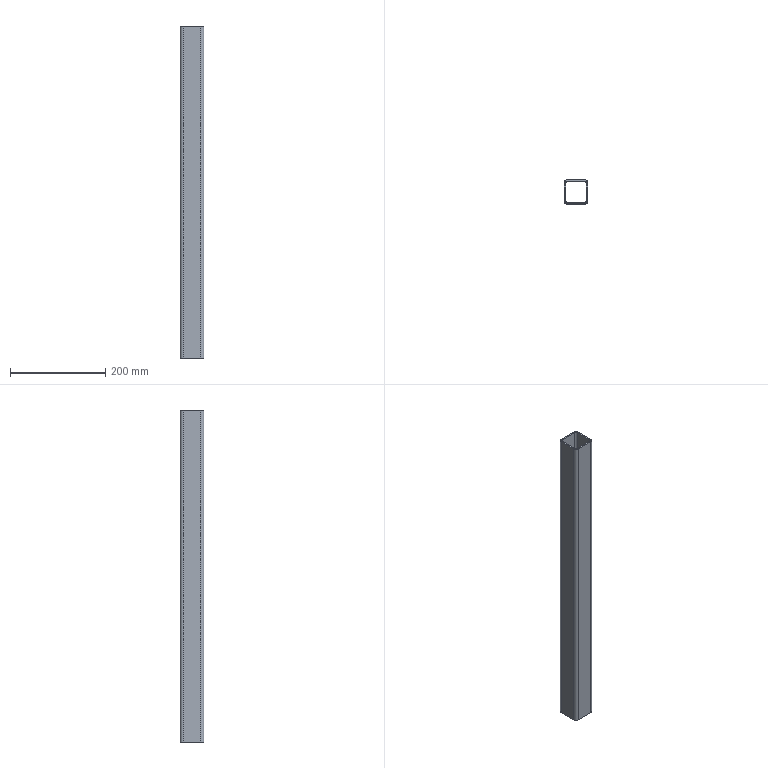Part | STEP file | JIS G 3466 50 x 50 x 3,2 1784904005805 | 1 solid | 18 faces | box 50 x 50 x 698.813 mm | volume 400189 mm3 | plane 10 | cylinder 8 | commonest cylinder face diameters 6.4 x4 12.8 x4
STEP:
#1=CARTESIAN_POINT('',(-18.6,-21.8,698.813));
#2=VERTEX_POINT('',#1);
#3=CARTESIAN_POINT('',(18.6,-21.8,698.813));
#4=VERTEX_POINT('',#3);
#5=CARTESIAN_POINT('',(9.3,-21.8,698.813));
#6=DIRECTION('',(1.,0.,0.));
#7=VECTOR('',#6,10.);
#8=LINE('',#5,#7);
#9=EDGE_CURVE('',#2,#4,#8,.T.);
#10=ORIENTED_EDGE('',*,*,#9,.T.);
#11=CARTESIAN_POINT('',(18.6,-21.8,0.));
#12=VERTEX_POINT('',#11);
#13=CARTESIAN_POINT('',(18.6,-21.8,0.));
#14=DIRECTION('',(0.,0.,1.));
#15=VECTOR('',#14,10.);
#16=LINE('',#13,#15);
#17=EDGE_CURVE('',#12,#4,#16,.T.);
#18=ORIENTED_EDGE('',*,*,#17,.F.);
#19=CARTESIAN_POINT('',(-18.6,-21.8,0.));
#20=VERTEX_POINT('',#19);
#21=CARTESIAN_POINT('',(9.3,-21.8,0.));
#22=DIRECTION('',(1.,0.,0.));
#23=VECTOR('',#22,10.);
#24=LINE('',#21,#23);
#25=EDGE_CURVE('',#20,#12,#24,.T.);
#26=ORIENTED_EDGE('',*,*,#25,.F.);
#27=CARTESIAN_POINT('',(-18.6,-21.8,0.));
#28=DIRECTION('',(0.,0.,1.));
#29=VECTOR('',#28,10.);
#30=LINE('',#27,#29);
#31=EDGE_CURVE('',#20,#2,#30,.T.);
#32=ORIENTED_EDGE('',*,*,#31,.T.);
#33=EDGE_LOOP('',(#10,#18,#26,#32));
#34=FACE_OUTER_BOUND('',#33,.T.);
#35=CARTESIAN_POINT('',(18.6,-21.8,0.));
#36=DIRECTION('',(0.,-1.,0.));
#37=DIRECTION('',(0.,0.,-1.));
#38=AXIS2_PLACEMENT_3D('',#35,#36,#37);
#39=PLANE('',#38);
#40=ADVANCED_FACE('',(#34),#39,.F.);
#41=CARTESIAN_POINT('',(21.8,-18.6,698.813));
#42=VERTEX_POINT('',#41);
#43=CARTESIAN_POINT('',(18.6,-18.6,698.813));
#44=DIRECTION('',(0.,0.,1.));
#45=DIRECTION('',(0.,1.,0.));
#46=AXIS2_PLACEMENT_3D('',#43,#44,#45);
#47=CIRCLE('',#46,3.2);
#48=EDGE_CURVE('',#4,#42,#47,.T.);
#49=ORIENTED_EDGE('',*,*,#48,.T.);
#50=CARTESIAN_POINT('',(21.8,-18.6,0.));
#51=VERTEX_POINT('',#50);
#52=CARTESIAN_POINT('',(21.8,-18.6,0.));
#53=DIRECTION('',(0.,0.,1.));
#54=VECTOR('',#53,10.);
#55=LINE('',#52,#54);
#56=EDGE_CURVE('',#51,#42,#55,.T.);
#57=ORIENTED_EDGE('',*,*,#56,.F.);
#58=CARTESIAN_POINT('',(18.6,-18.6,0.));
#59=DIRECTION('',(0.,0.,1.));
#60=DIRECTION('',(0.,1.,0.));
#61=AXIS2_PLACEMENT_3D('',#58,#59,#60);
#62=CIRCLE('',#61,3.2);
#63=EDGE_CURVE('',#12,#51,#62,.T.);
#64=ORIENTED_EDGE('',*,*,#63,.F.);
#65=ORIENTED_EDGE('',*,*,#17,.T.);
#66=EDGE_LOOP('',(#49,#57,#64,#65));
#67=FACE_OUTER_BOUND('',#66,.T.);
#68=CARTESIAN_POINT('',(18.6,-18.6,0.));
#69=DIRECTION('',(0.,0.,1.));
#70=DIRECTION('',(0.,1.,0.));
#71=AXIS2_PLACEMENT_3D('',#68,#69,#70);
#72=CYLINDRICAL_SURFACE('',#71,3.2);
#73=ADVANCED_FACE('',(#67),#72,.F.);
#74=CARTESIAN_POINT('',(21.8,18.6,698.813));
#75=VERTEX_POINT('',#74);
#76=CARTESIAN_POINT('',(21.8,9.3,698.813));
#77=DIRECTION('',(0.,1.,0.));
#78=VECTOR('',#77,10.);
#79=LINE('',#76,#78);
#80=EDGE_CURVE('',#42,#75,#79,.T.);
#81=ORIENTED_EDGE('',*,*,#80,.T.);
#82=CARTESIAN_POINT('',(21.8,18.6,0.));
#83=VERTEX_POINT('',#82);
#84=CARTESIAN_POINT('',(21.8,18.6,0.));
#85=DIRECTION('',(0.,0.,1.));
#86=VECTOR('',#85,10.);
#87=LINE('',#84,#86);
#88=EDGE_CURVE('',#83,#75,#87,.T.);
#89=ORIENTED_EDGE('',*,*,#88,.F.);
#90=CARTESIAN_POINT('',(21.8,9.3,0.));
#91=DIRECTION('',(0.,1.,0.));
#92=VECTOR('',#91,10.);
#93=LINE('',#90,#92);
#94=EDGE_CURVE('',#51,#83,#93,.T.);
#95=ORIENTED_EDGE('',*,*,#94,.F.);
#96=ORIENTED_EDGE('',*,*,#56,.T.);
#97=EDGE_LOOP('',(#81,#89,#95,#96));
#98=FACE_OUTER_BOUND('',#97,.T.);
#99=CARTESIAN_POINT('',(21.8,18.6,0.));
#100=DIRECTION('',(1.,0.,0.));
#101=DIRECTION('',(0.,0.,-1.));
#102=AXIS2_PLACEMENT_3D('',#99,#100,#101);
#103=PLANE('',#102);
#104=ADVANCED_FACE('',(#98),#103,.F.);
#105=CARTESIAN_POINT('',(18.6,21.8,698.813));
#106=VERTEX_POINT('',#105);
#107=CARTESIAN_POINT('',(18.6,18.6,698.813));
#108=DIRECTION('',(0.,0.,1.));
#109=DIRECTION('',(-1.,0.,0.));
#110=AXIS2_PLACEMENT_3D('',#107,#108,#109);
#111=CIRCLE('',#110,3.2);
#112=EDGE_CURVE('',#75,#106,#111,.T.);
#113=ORIENTED_EDGE('',*,*,#112,.T.);
#114=CARTESIAN_POINT('',(18.6,21.8,0.));
#115=VERTEX_POINT('',#114);
#116=CARTESIAN_POINT('',(18.6,21.8,0.));
#117=DIRECTION('',(0.,0.,1.));
#118=VECTOR('',#117,10.);
#119=LINE('',#116,#118);
#120=EDGE_CURVE('',#115,#106,#119,.T.);
#121=ORIENTED_EDGE('',*,*,#120,.F.);
#122=CARTESIAN_POINT('',(18.6,18.6,0.));
#123=DIRECTION('',(0.,0.,1.));
#124=DIRECTION('',(-1.,0.,0.));
#125=AXIS2_PLACEMENT_3D('',#122,#123,#124);
#126=CIRCLE('',#125,3.2);
#127=EDGE_CURVE('',#83,#115,#126,.T.);
#128=ORIENTED_EDGE('',*,*,#127,.F.);
#129=ORIENTED_EDGE('',*,*,#88,.T.);
#130=EDGE_LOOP('',(#113,#121,#128,#129));
#131=FACE_OUTER_BOUND('',#130,.T.);
#132=CARTESIAN_POINT('',(18.6,18.6,0.));
#133=DIRECTION('',(0.,0.,1.));
#134=DIRECTION('',(-1.,0.,0.));
#135=AXIS2_PLACEMENT_3D('',#132,#133,#134);
#136=CYLINDRICAL_SURFACE('',#135,3.2);
#137=ADVANCED_FACE('',(#131),#136,.F.);
#138=CARTESIAN_POINT('',(25.,18.6,698.813));
#139=VERTEX_POINT('',#138);
#140=CARTESIAN_POINT('',(25.,-18.6,698.813));
#141=VERTEX_POINT('',#140);
#142=CARTESIAN_POINT('',(25.,9.3,698.813));
#143=DIRECTION('',(0.,-1.,0.));
#144=VECTOR('',#143,10.);
#145=LINE('',#142,#144);
#146=EDGE_CURVE('',#139,#141,#145,.T.);
#147=ORIENTED_EDGE('',*,*,#146,.T.);
#148=CARTESIAN_POINT('',(25.,-18.6,0.));
#149=VERTEX_POINT('',#148);
#150=CARTESIAN_POINT('',(25.,-18.6,0.));
#151=DIRECTION('',(0.,0.,1.));
#152=VECTOR('',#151,10.);
#153=LINE('',#150,#152);
#154=EDGE_CURVE('',#149,#141,#153,.T.);
#155=ORIENTED_EDGE('',*,*,#154,.F.);
#156=CARTESIAN_POINT('',(25.,18.6,0.));
#157=VERTEX_POINT('',#156);
#158=CARTESIAN_POINT('',(25.,9.3,0.));
#159=DIRECTION('',(0.,-1.,0.));
#160=VECTOR('',#159,10.);
#161=LINE('',#158,#160);
#162=EDGE_CURVE('',#157,#149,#161,.T.);
#163=ORIENTED_EDGE('',*,*,#162,.F.);
#164=CARTESIAN_POINT('',(25.,18.6,0.));
#165=DIRECTION('',(0.,0.,1.));
#166=VECTOR('',#165,10.);
#167=LINE('',#164,#166);
#168=EDGE_CURVE('',#157,#139,#167,.T.);
#169=ORIENTED_EDGE('',*,*,#168,.T.);
#170=EDGE_LOOP('',(#147,#155,#163,#169));
#171=FACE_OUTER_BOUND('',#170,.T.);
#172=CARTESIAN_POINT('',(25.,18.6,0.));
#173=DIRECTION('',(1.,0.,0.));
#174=DIRECTION('',(0.,0.,-1.));
#175=AXIS2_PLACEMENT_3D('',#172,#173,#174);
#176=PLANE('',#175);
#177=ADVANCED_FACE('',(#171),#176,.T.);
#178=CARTESIAN_POINT('',(18.6,-25.,698.813));
#179=VERTEX_POINT('',#178);
#180=CARTESIAN_POINT('',(18.6,-18.6,698.813));
#181=DIRECTION('',(0.,0.,-1.));
#182=DIRECTION('',(0.,1.,0.));
#183=AXIS2_PLACEMENT_3D('',#180,#181,#182);
#184=CIRCLE('',#183,6.4);
#185=EDGE_CURVE('',#141,#179,#184,.T.);
#186=ORIENTED_EDGE('',*,*,#185,.T.);
#187=CARTESIAN_POINT('',(18.6,-25.,0.));
#188=VERTEX_POINT('',#187);
#189=CARTESIAN_POINT('',(18.6,-25.,0.));
#190=DIRECTION('',(0.,0.,1.));
#191=VECTOR('',#190,10.);
#192=LINE('',#189,#191);
#193=EDGE_CURVE('',#188,#179,#192,.T.);
#194=ORIENTED_EDGE('',*,*,#193,.F.);
#195=CARTESIAN_POINT('',(18.6,-18.6,0.));
#196=DIRECTION('',(0.,0.,-1.));
#197=DIRECTION('',(0.,1.,0.));
#198=AXIS2_PLACEMENT_3D('',#195,#196,#197);
#199=CIRCLE('',#198,6.4);
#200=EDGE_CURVE('',#149,#188,#199,.T.);
#201=ORIENTED_EDGE('',*,*,#200,.F.);
#202=ORIENTED_EDGE('',*,*,#154,.T.);
#203=EDGE_LOOP('',(#186,#194,#201,#202));
#204=FACE_OUTER_BOUND('',#203,.T.);
#205=CARTESIAN_POINT('',(18.6,-18.6,0.));
#206=DIRECTION('',(0.,0.,1.));
#207=DIRECTION('',(0.,1.,0.));
#208=AXIS2_PLACEMENT_3D('',#205,#206,#207);
#209=CYLINDRICAL_SURFACE('',#208,6.4);
#210=ADVANCED_FACE('',(#204),#209,.T.);
#211=CARTESIAN_POINT('',(-18.6,-25.,698.813));
#212=VERTEX_POINT('',#211);
#213=CARTESIAN_POINT('',(9.3,-25.,698.813));
#214=DIRECTION('',(-1.,0.,0.));
#215=VECTOR('',#214,10.);
#216=LINE('',#213,#215);
#217=EDGE_CURVE('',#179,#212,#216,.T.);
#218=ORIENTED_EDGE('',*,*,#217,.T.);
#219=CARTESIAN_POINT('',(-18.6,-25.,0.));
#220=VERTEX_POINT('',#219);
#221=CARTESIAN_POINT('',(-18.6,-25.,0.));
#222=DIRECTION('',(0.,0.,1.));
#223=VECTOR('',#222,10.);
#224=LINE('',#221,#223);
#225=EDGE_CURVE('',#220,#212,#224,.T.);
#226=ORIENTED_EDGE('',*,*,#225,.F.);
#227=CARTESIAN_POINT('',(9.3,-25.,0.));
#228=DIRECTION('',(-1.,0.,0.));
#229=VECTOR('',#228,10.);
#230=LINE('',#227,#229);
#231=EDGE_CURVE('',#188,#220,#230,.T.);
#232=ORIENTED_EDGE('',*,*,#231,.F.);
#233=ORIENTED_EDGE('',*,*,#193,.T.);
#234=EDGE_LOOP('',(#218,#226,#232,#233));
#235=FACE_OUTER_BOUND('',#234,.T.);
#236=CARTESIAN_POINT('',(18.6,-25.,0.));
#237=DIRECTION('',(0.,-1.,0.));
#238=DIRECTION('',(0.,0.,-1.));
#239=AXIS2_PLACEMENT_3D('',#236,#237,#238);
#240=PLANE('',#239);
#241=ADVANCED_FACE('',(#235),#240,.T.);
#242=CARTESIAN_POINT('',(-25.,-18.6,698.813));
#243=VERTEX_POINT('',#242);
#244=CARTESIAN_POINT('',(-18.6,-18.6,698.813));
#245=DIRECTION('',(0.,0.,-1.));
#246=DIRECTION('',(1.,0.,0.));
#247=AXIS2_PLACEMENT_3D('',#244,#245,#246);
#248=CIRCLE('',#247,6.4);
#249=EDGE_CURVE('',#212,#243,#248,.T.);
#250=ORIENTED_EDGE('',*,*,#249,.T.);
#251=CARTESIAN_POINT('',(-25.,-18.6,0.));
#252=VERTEX_POINT('',#251);
#253=CARTESIAN_POINT('',(-25.,-18.6,0.));
#254=DIRECTION('',(0.,0.,1.));
#255=VECTOR('',#254,10.);
#256=LINE('',#253,#255);
#257=EDGE_CURVE('',#252,#243,#256,.T.);
#258=ORIENTED_EDGE('',*,*,#257,.F.);
#259=CARTESIAN_POINT('',(-18.6,-18.6,0.));
#260=DIRECTION('',(0.,0.,-1.));
#261=DIRECTION('',(1.,0.,0.));
#262=AXIS2_PLACEMENT_3D('',#259,#260,#261);
#263=CIRCLE('',#262,6.4);
#264=EDGE_CURVE('',#220,#252,#263,.T.);
#265=ORIENTED_EDGE('',*,*,#264,.F.);
#266=ORIENTED_EDGE('',*,*,#225,.T.);
#267=EDGE_LOOP('',(#250,#258,#265,#266));
#268=FACE_OUTER_BOUND('',#267,.T.);
#269=CARTESIAN_POINT('',(-18.6,-18.6,0.));
#270=DIRECTION('',(0.,0.,1.));
#271=DIRECTION('',(1.,0.,0.));
#272=AXIS2_PLACEMENT_3D('',#269,#270,#271);
#273=CYLINDRICAL_SURFACE('',#272,6.4);
#274=ADVANCED_FACE('',(#268),#273,.T.);
#275=CARTESIAN_POINT('',(-18.6,21.8,698.813));
#276=VERTEX_POINT('',#275);
#277=CARTESIAN_POINT('',(-9.3,21.8,698.813));
#278=DIRECTION('',(-1.,0.,0.));
#279=VECTOR('',#278,10.);
#280=LINE('',#277,#279);
#281=EDGE_CURVE('',#106,#276,#280,.T.);
#282=ORIENTED_EDGE('',*,*,#281,.T.);
#283=CARTESIAN_POINT('',(-18.6,21.8,0.));
#284=VERTEX_POINT('',#283);
#285=CARTESIAN_POINT('',(-18.6,21.8,0.));
#286=DIRECTION('',(0.,0.,1.));
#287=VECTOR('',#286,10.);
#288=LINE('',#285,#287);
#289=EDGE_CURVE('',#284,#276,#288,.T.);
#290=ORIENTED_EDGE('',*,*,#289,.F.);
#291=CARTESIAN_POINT('',(-9.3,21.8,0.));
#292=DIRECTION('',(-1.,0.,0.));
#293=VECTOR('',#292,10.);
#294=LINE('',#291,#293);
#295=EDGE_CURVE('',#115,#284,#294,.T.);
#296=ORIENTED_EDGE('',*,*,#295,.F.);
#297=ORIENTED_EDGE('',*,*,#120,.T.);
#298=EDGE_LOOP('',(#282,#290,#296,#297));
#299=FACE_OUTER_BOUND('',#298,.T.);
#300=CARTESIAN_POINT('',(-18.6,21.8,0.));
#301=DIRECTION('',(0.,1.,0.));
#302=DIRECTION('',(0.,0.,1.));
#303=AXIS2_PLACEMENT_3D('',#300,#301,#302);
#304=PLANE('',#303);
#305=ADVANCED_FACE('',(#299),#304,.F.);
#306=CARTESIAN_POINT('',(-21.8,-18.6,698.813));
#307=VERTEX_POINT('',#306);
#308=CARTESIAN_POINT('',(-18.6,-18.6,698.813));
#309=DIRECTION('',(0.,0.,1.));
#310=DIRECTION('',(1.,0.,0.));
#311=AXIS2_PLACEMENT_3D('',#308,#309,#310);
#312=CIRCLE('',#311,3.2);
#313=EDGE_CURVE('',#307,#2,#312,.T.);
#314=ORIENTED_EDGE('',*,*,#313,.T.);
#315=ORIENTED_EDGE('',*,*,#31,.F.);
#316=CARTESIAN_POINT('',(-21.8,-18.6,0.));
#317=VERTEX_POINT('',#316);
#318=CARTESIAN_POINT('',(-18.6,-18.6,0.));
#319=DIRECTION('',(0.,0.,1.));
#320=DIRECTION('',(1.,0.,0.));
#321=AXIS2_PLACEMENT_3D('',#318,#319,#320);
#322=CIRCLE('',#321,3.2);
#323=EDGE_CURVE('',#317,#20,#322,.T.);
#324=ORIENTED_EDGE('',*,*,#323,.F.);
#325=CARTESIAN_POINT('',(-21.8,-18.6,0.));
#326=DIRECTION('',(0.,0.,1.));
#327=VECTOR('',#326,10.);
#328=LINE('',#325,#327);
#329=EDGE_CURVE('',#317,#307,#328,.T.);
#330=ORIENTED_EDGE('',*,*,#329,.T.);
#331=EDGE_LOOP('',(#314,#315,#324,#330));
#332=FACE_OUTER_BOUND('',#331,.T.);
#333=CARTESIAN_POINT('',(-18.6,-18.6,0.));
#334=DIRECTION('',(0.,0.,1.));
#335=DIRECTION('',(1.,0.,0.));
#336=AXIS2_PLACEMENT_3D('',#333,#334,#335);
#337=CYLINDRICAL_SURFACE('',#336,3.2);
#338=ADVANCED_FACE('',(#332),#337,.F.);
#339=CARTESIAN_POINT('',(-21.8,18.6,698.813));
#340=VERTEX_POINT('',#339);
#341=CARTESIAN_POINT('',(-21.8,-9.3,698.813));
#342=DIRECTION('',(0.,-1.,0.));
#343=VECTOR('',#342,10.);
#344=LINE('',#341,#343);
#345=EDGE_CURVE('',#340,#307,#344,.T.);
#346=ORIENTED_EDGE('',*,*,#345,.T.);
#347=ORIENTED_EDGE('',*,*,#329,.F.);
#348=CARTESIAN_POINT('',(-21.8,18.6,0.));
#349=VERTEX_POINT('',#348);
#350=CARTESIAN_POINT('',(-21.8,-9.3,0.));
#351=DIRECTION('',(0.,-1.,0.));
#352=VECTOR('',#351,10.);
#353=LINE('',#350,#352);
#354=EDGE_CURVE('',#349,#317,#353,.T.);
#355=ORIENTED_EDGE('',*,*,#354,.F.);
#356=CARTESIAN_POINT('',(-21.8,18.6,0.));
#357=DIRECTION('',(0.,0.,1.));
#358=VECTOR('',#357,10.);
#359=LINE('',#356,#358);
#360=EDGE_CURVE('',#349,#340,#359,.T.);
#361=ORIENTED_EDGE('',*,*,#360,.T.);
#362=EDGE_LOOP('',(#346,#347,#355,#361));
#363=FACE_OUTER_BOUND('',#362,.T.);
#364=CARTESIAN_POINT('',(-21.8,-18.6,0.));
#365=DIRECTION('',(-1.,0.,0.));
#366=DIRECTION('',(0.,0.,1.));
#367=AXIS2_PLACEMENT_3D('',#364,#365,#366);
#368=PLANE('',#367);
#369=ADVANCED_FACE('',(#363),#368,.F.);
#370=CARTESIAN_POINT('',(-18.6,18.6,698.813));
#371=DIRECTION('',(0.,0.,1.));
#372=DIRECTION('',(0.,-1.,0.));
#373=AXIS2_PLACEMENT_3D('',#370,#371,#372);
#374=CIRCLE('',#373,3.2);
#375=EDGE_CURVE('',#276,#340,#374,.T.);
#376=ORIENTED_EDGE('',*,*,#375,.T.);
#377=ORIENTED_EDGE('',*,*,#360,.F.);
#378=CARTESIAN_POINT('',(-18.6,18.6,0.));
#379=DIRECTION('',(0.,0.,1.));
#380=DIRECTION('',(0.,-1.,0.));
#381=AXIS2_PLACEMENT_3D('',#378,#379,#380);
#382=CIRCLE('',#381,3.2);
#383=EDGE_CURVE('',#284,#349,#382,.T.);
#384=ORIENTED_EDGE('',*,*,#383,.F.);
#385=ORIENTED_EDGE('',*,*,#289,.T.);
#386=EDGE_LOOP('',(#376,#377,#384,#385));
#387=FACE_OUTER_BOUND('',#386,.T.);
#388=CARTESIAN_POINT('',(-18.6,18.6,0.));
#389=DIRECTION('',(0.,0.,1.));
#390=DIRECTION('',(0.,-1.,0.));
#391=AXIS2_PLACEMENT_3D('',#388,#389,#390);
#392=CYLINDRICAL_SURFACE('',#391,3.2);
#393=ADVANCED_FACE('',(#387),#392,.F.);
#394=CARTESIAN_POINT('',(-25.,18.6,698.813));
#395=VERTEX_POINT('',#394);
#396=CARTESIAN_POINT('',(-25.,-9.3,698.813));
#397=DIRECTION('',(0.,1.,0.));
#398=VECTOR('',#397,10.);
#399=LINE('',#396,#398);
#400=EDGE_CURVE('',#243,#395,#399,.T.);
#401=ORIENTED_EDGE('',*,*,#400,.T.);
#402=CARTESIAN_POINT('',(-25.,18.6,0.));
#403=VERTEX_POINT('',#402);
#404=CARTESIAN_POINT('',(-25.,18.6,0.));
#405=DIRECTION('',(0.,0.,1.));
#406=VECTOR('',#405,10.);
#407=LINE('',#404,#406);
#408=EDGE_CURVE('',#403,#395,#407,.T.);
#409=ORIENTED_EDGE('',*,*,#408,.F.);
#410=CARTESIAN_POINT('',(-25.,-9.3,0.));
#411=DIRECTION('',(0.,1.,0.));
#412=VECTOR('',#411,10.);
#413=LINE('',#410,#412);
#414=EDGE_CURVE('',#252,#403,#413,.T.);
#415=ORIENTED_EDGE('',*,*,#414,.F.);
#416=ORIENTED_EDGE('',*,*,#257,.T.);
#417=EDGE_LOOP('',(#401,#409,#415,#416));
#418=FACE_OUTER_BOUND('',#417,.T.);
#419=CARTESIAN_POINT('',(-25.,-18.6,0.));
#420=DIRECTION('',(-1.,0.,0.));
#421=DIRECTION('',(0.,0.,1.));
#422=AXIS2_PLACEMENT_3D('',#419,#420,#421);
#423=PLANE('',#422);
#424=ADVANCED_FACE('',(#418),#423,.T.);
#425=CARTESIAN_POINT('',(-18.6,25.,698.813));
#426=VERTEX_POINT('',#425);
#427=CARTESIAN_POINT('',(-18.6,18.6,698.813));
#428=DIRECTION('',(0.,0.,-1.));
#429=DIRECTION('',(0.,-1.,0.));
#430=AXIS2_PLACEMENT_3D('',#427,#428,#429);
#431=CIRCLE('',#430,6.4);
#432=EDGE_CURVE('',#395,#426,#431,.T.);
#433=ORIENTED_EDGE('',*,*,#432,.T.);
#434=CARTESIAN_POINT('',(-18.6,25.,0.));
#435=VERTEX_POINT('',#434);
#436=CARTESIAN_POINT('',(-18.6,25.,0.));
#437=DIRECTION('',(0.,0.,1.));
#438=VECTOR('',#437,10.);
#439=LINE('',#436,#438);
#440=EDGE_CURVE('',#435,#426,#439,.T.);
#441=ORIENTED_EDGE('',*,*,#440,.F.);
#442=CARTESIAN_POINT('',(-18.6,18.6,0.));
#443=DIRECTION('',(0.,0.,-1.));
#444=DIRECTION('',(0.,-1.,0.));
#445=AXIS2_PLACEMENT_3D('',#442,#443,#444);
#446=CIRCLE('',#445,6.4);
#447=EDGE_CURVE('',#403,#435,#446,.T.);
#448=ORIENTED_EDGE('',*,*,#447,.F.);
#449=ORIENTED_EDGE('',*,*,#408,.T.);
#450=EDGE_LOOP('',(#433,#441,#448,#449));
#451=FACE_OUTER_BOUND('',#450,.T.);
#452=CARTESIAN_POINT('',(-18.6,18.6,0.));
#453=DIRECTION('',(0.,0.,1.));
#454=DIRECTION('',(0.,-1.,0.));
#455=AXIS2_PLACEMENT_3D('',#452,#453,#454);
#456=CYLINDRICAL_SURFACE('',#455,6.4);
#457=ADVANCED_FACE('',(#451),#456,.T.);
#458=CARTESIAN_POINT('',(18.6,25.,698.813));
#459=VERTEX_POINT('',#458);
#460=CARTESIAN_POINT('',(-9.3,25.,698.813));
#461=DIRECTION('',(1.,0.,0.));
#462=VECTOR('',#461,10.);
#463=LINE('',#460,#462);
#464=EDGE_CURVE('',#426,#459,#463,.T.);
#465=ORIENTED_EDGE('',*,*,#464,.T.);
#466=CARTESIAN_POINT('',(18.6,25.,0.));
#467=VERTEX_POINT('',#466);
#468=CARTESIAN_POINT('',(18.6,25.,0.));
#469=DIRECTION('',(0.,0.,1.));
#470=VECTOR('',#469,10.);
#471=LINE('',#468,#470);
#472=EDGE_CURVE('',#467,#459,#471,.T.);
#473=ORIENTED_EDGE('',*,*,#472,.F.);
#474=CARTESIAN_POINT('',(-9.3,25.,0.));
#475=DIRECTION('',(1.,0.,0.));
#476=VECTOR('',#475,10.);
#477=LINE('',#474,#476);
#478=EDGE_CURVE('',#435,#467,#477,.T.);
#479=ORIENTED_EDGE('',*,*,#478,.F.);
#480=ORIENTED_EDGE('',*,*,#440,.T.);
#481=EDGE_LOOP('',(#465,#473,#479,#480));
#482=FACE_OUTER_BOUND('',#481,.T.);
#483=CARTESIAN_POINT('',(-18.6,25.,0.));
#484=DIRECTION('',(0.,1.,0.));
#485=DIRECTION('',(0.,0.,1.));
#486=AXIS2_PLACEMENT_3D('',#483,#484,#485);
#487=PLANE('',#486);
#488=ADVANCED_FACE('',(#482),#487,.T.);
#489=CARTESIAN_POINT('',(18.6,18.6,698.813));
#490=DIRECTION('',(0.,0.,-1.));
#491=DIRECTION('',(-1.,0.,0.));
#492=AXIS2_PLACEMENT_3D('',#489,#490,#491);
#493=CIRCLE('',#492,6.4);
#494=EDGE_CURVE('',#459,#139,#493,.T.);
#495=ORIENTED_EDGE('',*,*,#494,.T.);
#496=ORIENTED_EDGE('',*,*,#168,.F.);
#497=CARTESIAN_POINT('',(18.6,18.6,0.));
#498=DIRECTION('',(0.,0.,-1.));
#499=DIRECTION('',(-1.,0.,0.));
#500=AXIS2_PLACEMENT_3D('',#497,#498,#499);
#501=CIRCLE('',#500,6.4);
#502=EDGE_CURVE('',#467,#157,#501,.T.);
#503=ORIENTED_EDGE('',*,*,#502,.F.);
#504=ORIENTED_EDGE('',*,*,#472,.T.);
#505=EDGE_LOOP('',(#495,#496,#503,#504));
#506=FACE_OUTER_BOUND('',#505,.T.);
#507=CARTESIAN_POINT('',(18.6,18.6,0.));
#508=DIRECTION('',(0.,0.,1.));
#509=DIRECTION('',(-1.,0.,0.));
#510=AXIS2_PLACEMENT_3D('',#507,#508,#509);
#511=CYLINDRICAL_SURFACE('',#510,6.4);
#512=ADVANCED_FACE('',(#506),#511,.T.);
#513=ORIENTED_EDGE('',*,*,#414,.T.);
#514=ORIENTED_EDGE('',*,*,#447,.T.);
#515=ORIENTED_EDGE('',*,*,#478,.T.);
#516=ORIENTED_EDGE('',*,*,#502,.T.);
#517=ORIENTED_EDGE('',*,*,#162,.T.);
#518=ORIENTED_EDGE('',*,*,#200,.T.);
#519=ORIENTED_EDGE('',*,*,#231,.T.);
#520=ORIENTED_EDGE('',*,*,#264,.T.);
#521=EDGE_LOOP('',(#513,#514,#515,#516,#517,#518,#519,#520));
#522=FACE_OUTER_BOUND('',#521,.T.);
#523=ORIENTED_EDGE('',*,*,#295,.T.);
#524=ORIENTED_EDGE('',*,*,#383,.T.);
#525=ORIENTED_EDGE('',*,*,#354,.T.);
#526=ORIENTED_EDGE('',*,*,#323,.T.);
#527=ORIENTED_EDGE('',*,*,#25,.T.);
#528=ORIENTED_EDGE('',*,*,#63,.T.);
#529=ORIENTED_EDGE('',*,*,#94,.T.);
#530=ORIENTED_EDGE('',*,*,#127,.T.);
#531=EDGE_LOOP('',(#523,#524,#525,#526,#527,#528,#529,#530));
#532=FACE_BOUND('',#531,.T.);
#533=CARTESIAN_POINT('',(0.,0.,0.));
#534=DIRECTION('',(0.,0.,1.));
#535=DIRECTION('',(1.,0.,0.));
#536=AXIS2_PLACEMENT_3D('',#533,#534,#535);
#537=PLANE('',#536);
#538=ADVANCED_FACE('',(#522,#532),#537,.F.);
#539=ORIENTED_EDGE('',*,*,#400,.F.);
#540=ORIENTED_EDGE('',*,*,#249,.F.);
#541=ORIENTED_EDGE('',*,*,#217,.F.);
#542=ORIENTED_EDGE('',*,*,#185,.F.);
#543=ORIENTED_EDGE('',*,*,#146,.F.);
#544=ORIENTED_EDGE('',*,*,#494,.F.);
#545=ORIENTED_EDGE('',*,*,#464,.F.);
#546=ORIENTED_EDGE('',*,*,#432,.F.);
#547=EDGE_LOOP('',(#539,#540,#541,#542,#543,#544,#545,#546));
#548=FACE_OUTER_BOUND('',#547,.T.);
#549=ORIENTED_EDGE('',*,*,#281,.F.);
#550=ORIENTED_EDGE('',*,*,#112,.F.);
#551=ORIENTED_EDGE('',*,*,#80,.F.);
#552=ORIENTED_EDGE('',*,*,#48,.F.);
#553=ORIENTED_EDGE('',*,*,#9,.F.);
#554=ORIENTED_EDGE('',*,*,#313,.F.);
#555=ORIENTED_EDGE('',*,*,#345,.F.);
#556=ORIENTED_EDGE('',*,*,#375,.F.);
#557=EDGE_LOOP('',(#549,#550,#551,#552,#553,#554,#555,#556));
#558=FACE_BOUND('',#557,.T.);
#559=CARTESIAN_POINT('',(0.,0.,698.813));
#560=DIRECTION('',(0.,0.,1.));
#561=DIRECTION('',(1.,0.,0.));
#562=AXIS2_PLACEMENT_3D('',#559,#560,#561);
#563=PLANE('',#562);
#564=ADVANCED_FACE('',(#548,#558),#563,.T.);
#565=CLOSED_SHELL('',(#40,#73,#104,#137,#177,#210,#241,#274,#305,#338,#369,#393,#424,#457,#488,#512,#538,#564));
#566=MANIFOLD_SOLID_BREP('',#565);
#567=(LENGTH_UNIT()NAMED_UNIT(*)SI_UNIT(.MILLI.,.METRE.));
#568=UNCERTAINTY_MEASURE_WITH_UNIT(LENGTH_MEASURE(0.01),#567,'','');
#569=(NAMED_UNIT(*)PLANE_ANGLE_UNIT()SI_UNIT($,.RADIAN.));
#570=(NAMED_UNIT(*)SI_UNIT($,.STERADIAN.)SOLID_ANGLE_UNIT());
#571=(GEOMETRIC_REPRESENTATION_CONTEXT(3)GLOBAL_UNCERTAINTY_ASSIGNED_CONTEXT((#568))GLOBAL_UNIT_ASSIGNED_CONTEXT((#567,#569,#570))REPRESENTATION_CONTEXT('',''));
#572=ADVANCED_BREP_SHAPE_REPRESENTATION('',(#566),#571);